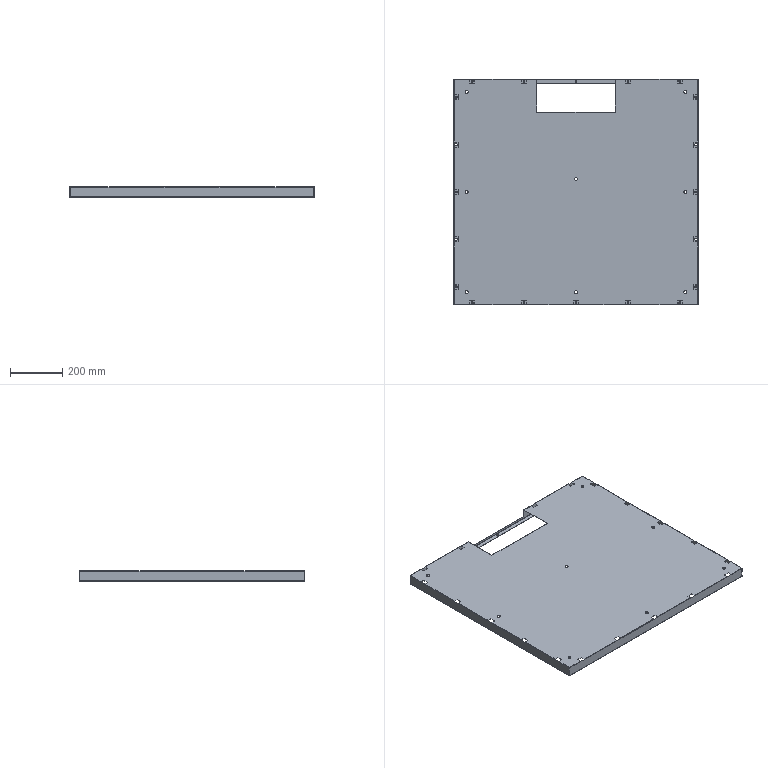Part | 1 solid | 376 faces | box 939 x 869 x 40 mm | volume 955606 mm3 | plane 238 | cylinder 122 | spline 16 | commonest cylinder face diameters 7 x50 0.4 x28 2.4 x28 11 x16